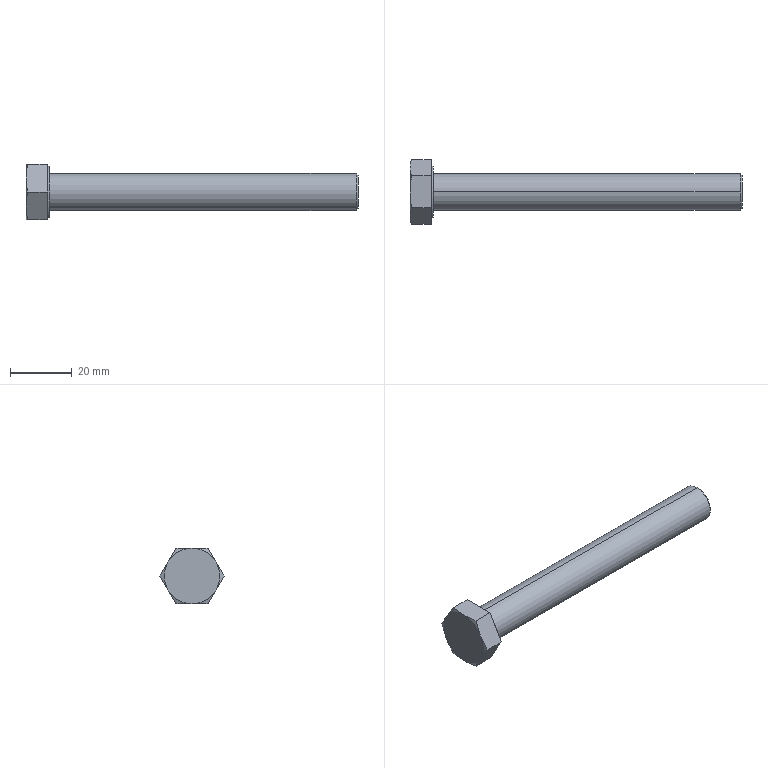Part | STEP file | GBT 5781#Hex head bolt fully threaded_M12×100-zinc plated | 1 solid | 22 faces | box 107.5 x 20.785 x 18 mm | volume 13373 mm3 | cone 10 | plane 10 | cylinder 2 | commonest cylinder face diameters 12 x2
STEP:
#1=CARTESIAN_POINT('',(107.5,0.,-5.4));
#2=VERTEX_POINT('',#1);
#3=CARTESIAN_POINT('',(107.5,0.,5.4));
#4=VERTEX_POINT('',#3);
#5=CARTESIAN_POINT('',(107.5,0.,0.));
#6=DIRECTION('',(1.,0.,0.));
#7=DIRECTION('',(0.,0.,-1.));
#8=AXIS2_PLACEMENT_3D('',#5,#6,#7);
#9=CIRCLE('',#8,5.4);
#10=EDGE_CURVE('',#2,#4,#9,.T.);
#11=ORIENTED_EDGE('',*,*,#10,.F.);
#12=CARTESIAN_POINT('',(106.9,0.,-6.));
#13=VERTEX_POINT('',#12);
#14=CARTESIAN_POINT('',(107.5,0.,-5.4));
#15=DIRECTION('',(-0.7071,0.,-0.7071));
#16=VECTOR('',#15,1000.);
#17=LINE('',#14,#16);
#18=EDGE_CURVE('',#2,#13,#17,.T.);
#19=ORIENTED_EDGE('',*,*,#18,.T.);
#20=CARTESIAN_POINT('',(106.9,0.,6.));
#21=VERTEX_POINT('',#20);
#22=CARTESIAN_POINT('',(106.9,0.,0.));
#23=DIRECTION('',(-1.,0.,0.));
#24=DIRECTION('',(0.,0.,-1.));
#25=AXIS2_PLACEMENT_3D('',#22,#23,#24);
#26=CIRCLE('',#25,6.);
#27=EDGE_CURVE('',#21,#13,#26,.T.);
#28=ORIENTED_EDGE('',*,*,#27,.F.);
#29=CARTESIAN_POINT('',(107.5,0.,5.4));
#30=DIRECTION('',(-0.7071,0.,0.7071));
#31=VECTOR('',#30,1000.);
#32=LINE('',#29,#31);
#33=EDGE_CURVE('',#4,#21,#32,.T.);
#34=ORIENTED_EDGE('',*,*,#33,.F.);
#35=EDGE_LOOP('',(#11,#19,#28,#34));
#36=FACE_OUTER_BOUND('',#35,.T.);
#37=CARTESIAN_POINT('',(107.5,0.,0.));
#38=DIRECTION('',(-1.,0.,0.));
#39=DIRECTION('',(0.,0.,1.));
#40=AXIS2_PLACEMENT_3D('',#37,#38,#39);
#41=CONICAL_SURFACE('',#40,5.4,0.7854);
#42=ADVANCED_FACE('',(#36),#41,.T.);
#43=ORIENTED_EDGE('',*,*,#27,.T.);
#44=CARTESIAN_POINT('',(7.5,0.,-6.));
#45=VERTEX_POINT('',#44);
#46=CARTESIAN_POINT('',(107.5,0.,-6.));
#47=DIRECTION('',(-1.,0.,0.));
#48=VECTOR('',#47,1000.);
#49=LINE('',#46,#48);
#50=EDGE_CURVE('',#13,#45,#49,.T.);
#51=ORIENTED_EDGE('',*,*,#50,.T.);
#52=CARTESIAN_POINT('',(7.5,0.,6.));
#53=VERTEX_POINT('',#52);
#54=CARTESIAN_POINT('',(7.5,0.,0.));
#55=DIRECTION('',(1.,0.,0.));
#56=DIRECTION('',(0.,0.,-1.));
#57=AXIS2_PLACEMENT_3D('',#54,#55,#56);
#58=CIRCLE('',#57,6.);
#59=EDGE_CURVE('',#45,#53,#58,.T.);
#60=ORIENTED_EDGE('',*,*,#59,.T.);
#61=CARTESIAN_POINT('',(107.5,0.,6.));
#62=DIRECTION('',(-1.,0.,0.));
#63=VECTOR('',#62,1000.);
#64=LINE('',#61,#63);
#65=EDGE_CURVE('',#21,#53,#64,.T.);
#66=ORIENTED_EDGE('',*,*,#65,.F.);
#67=EDGE_LOOP('',(#43,#51,#60,#66));
#68=FACE_OUTER_BOUND('',#67,.T.);
#69=CARTESIAN_POINT('',(107.5,0.,0.));
#70=DIRECTION('',(-1.,0.,0.));
#71=DIRECTION('',(0.,0.,1.));
#72=AXIS2_PLACEMENT_3D('',#69,#70,#71);
#73=CYLINDRICAL_SURFACE('',#72,6.);
#74=ADVANCED_FACE('',(#68),#73,.T.);
#75=CARTESIAN_POINT('',(7.5,0.,8.235));
#76=VERTEX_POINT('',#75);
#77=CARTESIAN_POINT('',(7.5,0.,-8.235));
#78=VERTEX_POINT('',#77);
#79=CARTESIAN_POINT('',(7.5,0.,0.));
#80=DIRECTION('',(-1.,0.,0.));
#81=DIRECTION('',(0.,0.,1.));
#82=AXIS2_PLACEMENT_3D('',#79,#80,#81);
#83=CIRCLE('',#82,8.235);
#84=EDGE_CURVE('',#76,#78,#83,.T.);
#85=ORIENTED_EDGE('',*,*,#84,.T.);
#86=CARTESIAN_POINT('',(6.9,0.,-8.835));
#87=VERTEX_POINT('',#86);
#88=CARTESIAN_POINT('',(6.9,0.,-8.835));
#89=DIRECTION('',(-0.7071,0.,-0.7071));
#90=VECTOR('',#89,1000.);
#91=LINE('',#88,#90);
#92=EDGE_CURVE('',#78,#87,#91,.T.);
#93=ORIENTED_EDGE('',*,*,#92,.T.);
#94=CARTESIAN_POINT('',(6.9,0.,8.835));
#95=VERTEX_POINT('',#94);
#96=CARTESIAN_POINT('',(6.9,0.,0.));
#97=DIRECTION('',(-1.,0.,0.));
#98=DIRECTION('',(0.,0.,1.));
#99=AXIS2_PLACEMENT_3D('',#96,#97,#98);
#100=CIRCLE('',#99,8.835);
#101=EDGE_CURVE('',#95,#87,#100,.T.);
#102=ORIENTED_EDGE('',*,*,#101,.F.);
#103=CARTESIAN_POINT('',(6.9,0.,8.835));
#104=DIRECTION('',(-0.7071,0.,0.7071));
#105=VECTOR('',#104,1000.);
#106=LINE('',#103,#105);
#107=EDGE_CURVE('',#76,#95,#106,.T.);
#108=ORIENTED_EDGE('',*,*,#107,.F.);
#109=EDGE_LOOP('',(#85,#93,#102,#108));
#110=FACE_OUTER_BOUND('',#109,.T.);
#111=CARTESIAN_POINT('',(6.9,0.,0.));
#112=DIRECTION('',(-1.,0.,0.));
#113=DIRECTION('',(0.,0.,1.));
#114=AXIS2_PLACEMENT_3D('',#111,#112,#113);
#115=CONICAL_SURFACE('',#114,8.835,0.7854);
#116=ADVANCED_FACE('',(#110),#115,.T.);
#117=ORIENTED_EDGE('',*,*,#84,.F.);
#118=CARTESIAN_POINT('',(7.5,0.,0.));
#119=DIRECTION('',(-1.,0.,0.));
#120=DIRECTION('',(0.,0.,1.));
#121=AXIS2_PLACEMENT_3D('',#118,#119,#120);
#122=CIRCLE('',#121,8.235);
#123=EDGE_CURVE('',#78,#76,#122,.T.);
#124=ORIENTED_EDGE('',*,*,#123,.F.);
#125=EDGE_LOOP('',(#117,#124));
#126=FACE_OUTER_BOUND('',#125,.T.);
#127=CARTESIAN_POINT('',(7.5,0.,0.));
#128=DIRECTION('',(1.,0.,0.));
#129=DIRECTION('',(0.,0.,-1.));
#130=AXIS2_PLACEMENT_3D('',#127,#128,#129);
#131=CIRCLE('',#130,6.);
#132=EDGE_CURVE('',#53,#45,#131,.T.);
#133=ORIENTED_EDGE('',*,*,#132,.F.);
#134=ORIENTED_EDGE('',*,*,#59,.F.);
#135=EDGE_LOOP('',(#133,#134));
#136=FACE_BOUND('',#135,.T.);
#137=CARTESIAN_POINT('',(7.5,-10.392,0.));
#138=DIRECTION('',(1.,0.,0.));
#139=DIRECTION('',(0.,0.,-1.));
#140=AXIS2_PLACEMENT_3D('',#137,#138,#139);
#141=PLANE('',#140);
#142=ADVANCED_FACE('',(#126,#136),#141,.T.);
#143=CARTESIAN_POINT('',(0.5068,-10.392,0.));
#144=VERTEX_POINT('',#143);
#145=CARTESIAN_POINT('',(0.,-7.794,4.5));
#146=VERTEX_POINT('',#145);
#147=CARTESIAN_POINT('',(0.5068,-10.392,0.));
#148=CARTESIAN_POINT('',(0.3492,-9.959,0.75));
#149=CARTESIAN_POINT('',(0.2212,-9.526,1.5));
#150=CARTESIAN_POINT('',(0.04634,-8.66,3.));
#151=CARTESIAN_POINT('',(0.,-8.227,3.75));
#152=CARTESIAN_POINT('',(0.,-7.794,4.5));
#153=B_SPLINE_CURVE_WITH_KNOTS('',3,(#147,#148,#149,#150,#151,#152),.UNSPECIFIED.,.F.,.F.,(4,2,4),(0.000000231,0.002598,0.005196),.UNSPECIFIED.);
#154=EDGE_CURVE('',#144,#146,#153,.T.);
#155=ORIENTED_EDGE('',*,*,#154,.F.);
#156=CARTESIAN_POINT('',(6.9,-10.392,0.));
#157=VERTEX_POINT('',#156);
#158=CARTESIAN_POINT('',(7.5,-10.392,0.));
#159=DIRECTION('',(-1.,0.,0.));
#160=VECTOR('',#159,1000.);
#161=LINE('',#158,#160);
#162=EDGE_CURVE('',#157,#144,#161,.T.);
#163=ORIENTED_EDGE('',*,*,#162,.F.);
#164=CARTESIAN_POINT('',(6.9,-5.196,9.));
#165=VERTEX_POINT('',#164);
#166=CARTESIAN_POINT('',(6.9,-5.196,9.));
#167=DIRECTION('',(0.,-0.5,-0.866));
#168=VECTOR('',#167,1000.);
#169=LINE('',#166,#168);
#170=EDGE_CURVE('',#165,#157,#169,.T.);
#171=ORIENTED_EDGE('',*,*,#170,.F.);
#172=CARTESIAN_POINT('',(0.5068,-5.196,9.));
#173=VERTEX_POINT('',#172);
#174=CARTESIAN_POINT('',(7.5,-5.196,9.));
#175=DIRECTION('',(-1.,0.,0.));
#176=VECTOR('',#175,1000.);
#177=LINE('',#174,#176);
#178=EDGE_CURVE('',#165,#173,#177,.T.);
#179=ORIENTED_EDGE('',*,*,#178,.T.);
#180=CARTESIAN_POINT('',(0.,-7.794,4.5));
#181=CARTESIAN_POINT('',(0.,-7.361,5.25));
#182=CARTESIAN_POINT('',(0.04634,-6.928,6.));
#183=CARTESIAN_POINT('',(0.2212,-6.062,7.5));
#184=CARTESIAN_POINT('',(0.3492,-5.629,8.25));
#185=CARTESIAN_POINT('',(0.5068,-5.196,9.));
#186=B_SPLINE_CURVE_WITH_KNOTS('',3,(#180,#181,#182,#183,#184,#185),.UNSPECIFIED.,.F.,.F.,(4,2,4),(0.005196,0.007794,0.01039),.UNSPECIFIED.);
#187=EDGE_CURVE('',#146,#173,#186,.T.);
#188=ORIENTED_EDGE('',*,*,#187,.F.);
#189=EDGE_LOOP('',(#155,#163,#171,#179,#188));
#190=FACE_OUTER_BOUND('',#189,.T.);
#191=CARTESIAN_POINT('',(7.5,-5.196,9.));
#192=DIRECTION('',(0.,0.866,-0.5));
#193=DIRECTION('',(0.,0.5,0.866));
#194=AXIS2_PLACEMENT_3D('',#191,#192,#193);
#195=PLANE('',#194);
#196=ADVANCED_FACE('',(#190),#195,.F.);
#197=CARTESIAN_POINT('',(0.5068,-5.196,-9.));
#198=VERTEX_POINT('',#197);
#199=CARTESIAN_POINT('',(0.,-7.794,-4.5));
#200=VERTEX_POINT('',#199);
#201=CARTESIAN_POINT('',(0.5068,-5.196,-9.));
#202=CARTESIAN_POINT('',(0.3492,-5.629,-8.25));
#203=CARTESIAN_POINT('',(0.2212,-6.062,-7.5));
#204=CARTESIAN_POINT('',(0.04634,-6.928,-6.));
#205=CARTESIAN_POINT('',(0.,-7.361,-5.25));
#206=CARTESIAN_POINT('',(0.,-7.794,-4.5));
#207=B_SPLINE_CURVE_WITH_KNOTS('',3,(#201,#202,#203,#204,#205,#206),.UNSPECIFIED.,.F.,.F.,(4,2,4),(0.000000231,0.002598,0.005196),.UNSPECIFIED.);
#208=EDGE_CURVE('',#198,#200,#207,.T.);
#209=ORIENTED_EDGE('',*,*,#208,.F.);
#210=CARTESIAN_POINT('',(6.9,-5.196,-9.));
#211=VERTEX_POINT('',#210);
#212=CARTESIAN_POINT('',(7.5,-5.196,-9.));
#213=DIRECTION('',(-1.,0.,0.));
#214=VECTOR('',#213,1000.);
#215=LINE('',#212,#214);
#216=EDGE_CURVE('',#211,#198,#215,.T.);
#217=ORIENTED_EDGE('',*,*,#216,.F.);
#218=CARTESIAN_POINT('',(6.9,-10.392,0.));
#219=DIRECTION('',(0.,0.5,-0.866));
#220=VECTOR('',#219,1000.);
#221=LINE('',#218,#220);
#222=EDGE_CURVE('',#157,#211,#221,.T.);
#223=ORIENTED_EDGE('',*,*,#222,.F.);
#224=ORIENTED_EDGE('',*,*,#162,.T.);
#225=CARTESIAN_POINT('',(0.,-7.794,-4.5));
#226=CARTESIAN_POINT('',(0.,-8.227,-3.75));
#227=CARTESIAN_POINT('',(0.04634,-8.66,-3.));
#228=CARTESIAN_POINT('',(0.2212,-9.526,-1.5));
#229=CARTESIAN_POINT('',(0.3492,-9.959,-0.75));
#230=CARTESIAN_POINT('',(0.5068,-10.392,0.));
#231=B_SPLINE_CURVE_WITH_KNOTS('',3,(#225,#226,#227,#228,#229,#230),.UNSPECIFIED.,.F.,.F.,(4,2,4),(0.005196,0.007794,0.01039),.UNSPECIFIED.);
#232=EDGE_CURVE('',#200,#144,#231,.T.);
#233=ORIENTED_EDGE('',*,*,#232,.F.);
#234=EDGE_LOOP('',(#209,#217,#223,#224,#233));
#235=FACE_OUTER_BOUND('',#234,.T.);
#236=CARTESIAN_POINT('',(7.5,-10.392,0.));
#237=DIRECTION('',(0.,0.866,0.5));
#238=DIRECTION('',(0.,-0.5,0.866));
#239=AXIS2_PLACEMENT_3D('',#236,#237,#238);
#240=PLANE('',#239);
#241=ADVANCED_FACE('',(#235),#240,.F.);
#242=CARTESIAN_POINT('',(0.5068,5.196,-9.));
#243=VERTEX_POINT('',#242);
#244=CARTESIAN_POINT('',(0.,0.,-9.));
#245=VERTEX_POINT('',#244);
#246=CARTESIAN_POINT('',(0.5068,5.196,-9.));
#247=CARTESIAN_POINT('',(0.3496,4.332,-9.));
#248=CARTESIAN_POINT('',(0.2215,3.467,-9.));
#249=CARTESIAN_POINT('',(0.04652,1.735,-9.));
#250=CARTESIAN_POINT('',(0.,0.8678,-9.));
#251=CARTESIAN_POINT('',(0.,0.,-9.));
#252=B_SPLINE_CURVE_WITH_KNOTS('',3,(#246,#247,#248,#249,#250,#251),.UNSPECIFIED.,.F.,.F.,(4,2,4),(0.01874,0.02136,0.02398),.UNSPECIFIED.);
#253=EDGE_CURVE('',#243,#245,#252,.T.);
#254=ORIENTED_EDGE('',*,*,#253,.F.);
#255=CARTESIAN_POINT('',(6.9,5.196,-9.));
#256=VERTEX_POINT('',#255);
#257=CARTESIAN_POINT('',(7.5,5.196,-9.));
#258=DIRECTION('',(-1.,0.,0.));
#259=VECTOR('',#258,1000.);
#260=LINE('',#257,#259);
#261=EDGE_CURVE('',#256,#243,#260,.T.);
#262=ORIENTED_EDGE('',*,*,#261,.F.);
#263=CARTESIAN_POINT('',(6.9,-5.196,-9.));
#264=DIRECTION('',(0.,1.,0.));
#265=VECTOR('',#264,1000.);
#266=LINE('',#263,#265);
#267=EDGE_CURVE('',#211,#256,#266,.T.);
#268=ORIENTED_EDGE('',*,*,#267,.F.);
#269=ORIENTED_EDGE('',*,*,#216,.T.);
#270=CARTESIAN_POINT('',(0.,0.,-9.));
#271=CARTESIAN_POINT('',(0.,-0.8653,-9.));
#272=CARTESIAN_POINT('',(0.04627,-1.732,-9.));
#273=CARTESIAN_POINT('',(0.2214,-3.466,-9.));
#274=CARTESIAN_POINT('',(0.3502,-4.336,-9.));
#275=CARTESIAN_POINT('',(0.5068,-5.196,-9.));
#276=B_SPLINE_CURVE_WITH_KNOTS('',3,(#270,#271,#272,#273,#274,#275),.UNSPECIFIED.,.F.,.F.,(4,2,4),(0.02398,0.02659,0.0292),.UNSPECIFIED.);
#277=EDGE_CURVE('',#245,#198,#276,.T.);
#278=ORIENTED_EDGE('',*,*,#277,.F.);
#279=EDGE_LOOP('',(#254,#262,#268,#269,#278));
#280=FACE_OUTER_BOUND('',#279,.T.);
#281=CARTESIAN_POINT('',(7.5,-5.196,-9.));
#282=DIRECTION('',(0.,0.,1.));
#283=DIRECTION('',(1.,0.,0.));
#284=AXIS2_PLACEMENT_3D('',#281,#282,#283);
#285=PLANE('',#284);
#286=ADVANCED_FACE('',(#280),#285,.F.);
#287=CARTESIAN_POINT('',(0.5068,10.392,0.));
#288=VERTEX_POINT('',#287);
#289=CARTESIAN_POINT('',(0.,7.794,-4.5));
#290=VERTEX_POINT('',#289);
#291=CARTESIAN_POINT('',(0.5068,10.392,0.));
#292=CARTESIAN_POINT('',(0.3492,9.959,-0.75));
#293=CARTESIAN_POINT('',(0.2212,9.526,-1.5));
#294=CARTESIAN_POINT('',(0.04634,8.66,-3.));
#295=CARTESIAN_POINT('',(0.,8.227,-3.75));
#296=CARTESIAN_POINT('',(0.,7.794,-4.5));
#297=B_SPLINE_CURVE_WITH_KNOTS('',3,(#291,#292,#293,#294,#295,#296),.UNSPECIFIED.,.F.,.F.,(4,2,4),(0.000000231,0.002598,0.005196),.UNSPECIFIED.);
#298=EDGE_CURVE('',#288,#290,#297,.T.);
#299=ORIENTED_EDGE('',*,*,#298,.F.);
#300=CARTESIAN_POINT('',(6.9,10.392,0.));
#301=VERTEX_POINT('',#300);
#302=CARTESIAN_POINT('',(7.5,10.392,0.));
#303=DIRECTION('',(-1.,0.,0.));
#304=VECTOR('',#303,1000.);
#305=LINE('',#302,#304);
#306=EDGE_CURVE('',#301,#288,#305,.T.);
#307=ORIENTED_EDGE('',*,*,#306,.F.);
#308=CARTESIAN_POINT('',(6.9,5.196,-9.));
#309=DIRECTION('',(0.,0.5,0.866));
#310=VECTOR('',#309,1000.);
#311=LINE('',#308,#310);
#312=EDGE_CURVE('',#256,#301,#311,.T.);
#313=ORIENTED_EDGE('',*,*,#312,.F.);
#314=ORIENTED_EDGE('',*,*,#261,.T.);
#315=CARTESIAN_POINT('',(0.,7.794,-4.5));
#316=CARTESIAN_POINT('',(0.,7.361,-5.25));
#317=CARTESIAN_POINT('',(0.04634,6.928,-6.));
#318=CARTESIAN_POINT('',(0.2212,6.062,-7.5));
#319=CARTESIAN_POINT('',(0.3492,5.629,-8.25));
#320=CARTESIAN_POINT('',(0.5068,5.196,-9.));
#321=B_SPLINE_CURVE_WITH_KNOTS('',3,(#315,#316,#317,#318,#319,#320),.UNSPECIFIED.,.F.,.F.,(4,2,4),(0.005196,0.007794,0.01039),.UNSPECIFIED.);
#322=EDGE_CURVE('',#290,#243,#321,.T.);
#323=ORIENTED_EDGE('',*,*,#322,.F.);
#324=EDGE_LOOP('',(#299,#307,#313,#314,#323));
#325=FACE_OUTER_BOUND('',#324,.T.);
#326=CARTESIAN_POINT('',(7.5,5.196,-9.));
#327=DIRECTION('',(0.,-0.866,0.5));
#328=DIRECTION('',(0.,-0.5,-0.866));
#329=AXIS2_PLACEMENT_3D('',#326,#327,#328);
#330=PLANE('',#329);
#331=ADVANCED_FACE('',(#325),#330,.F.);
#332=CARTESIAN_POINT('',(0.5068,5.196,9.));
#333=VERTEX_POINT('',#332);
#334=CARTESIAN_POINT('',(0.,7.794,4.5));
#335=VERTEX_POINT('',#334);
#336=CARTESIAN_POINT('',(0.5068,5.196,9.));
#337=CARTESIAN_POINT('',(0.3492,5.629,8.25));
#338=CARTESIAN_POINT('',(0.2212,6.062,7.5));
#339=CARTESIAN_POINT('',(0.04634,6.928,6.));
#340=CARTESIAN_POINT('',(0.,7.361,5.25));
#341=CARTESIAN_POINT('',(0.,7.794,4.5));
#342=B_SPLINE_CURVE_WITH_KNOTS('',3,(#336,#337,#338,#339,#340,#341),.UNSPECIFIED.,.F.,.F.,(4,2,4),(0.000000231,0.002598,0.005196),.UNSPECIFIED.);
#343=EDGE_CURVE('',#333,#335,#342,.T.);
#344=ORIENTED_EDGE('',*,*,#343,.F.);
#345=CARTESIAN_POINT('',(6.9,5.196,9.));
#346=VERTEX_POINT('',#345);
#347=CARTESIAN_POINT('',(7.5,5.196,9.));
#348=DIRECTION('',(-1.,0.,0.));
#349=VECTOR('',#348,1000.);
#350=LINE('',#347,#349);
#351=EDGE_CURVE('',#346,#333,#350,.T.);
#352=ORIENTED_EDGE('',*,*,#351,.F.);
#353=CARTESIAN_POINT('',(6.9,10.392,0.));
#354=DIRECTION('',(0.,-0.5,0.866));
#355=VECTOR('',#354,1000.);
#356=LINE('',#353,#355);
#357=EDGE_CURVE('',#301,#346,#356,.T.);
#358=ORIENTED_EDGE('',*,*,#357,.F.);
#359=ORIENTED_EDGE('',*,*,#306,.T.);
#360=CARTESIAN_POINT('',(0.,7.794,4.5));
#361=CARTESIAN_POINT('',(0.,8.227,3.75));
#362=CARTESIAN_POINT('',(0.04634,8.66,3.));
#363=CARTESIAN_POINT('',(0.2212,9.526,1.5));
#364=CARTESIAN_POINT('',(0.3492,9.959,0.75));
#365=CARTESIAN_POINT('',(0.5068,10.392,0.));
#366=B_SPLINE_CURVE_WITH_KNOTS('',3,(#360,#361,#362,#363,#364,#365),.UNSPECIFIED.,.F.,.F.,(4,2,4),(0.005196,0.007794,0.01039),.UNSPECIFIED.);
#367=EDGE_CURVE('',#335,#288,#366,.T.);
#368=ORIENTED_EDGE('',*,*,#367,.F.);
#369=EDGE_LOOP('',(#344,#352,#358,#359,#368));
#370=FACE_OUTER_BOUND('',#369,.T.);
#371=CARTESIAN_POINT('',(7.5,10.392,0.));
#372=DIRECTION('',(0.,-0.866,-0.5));
#373=DIRECTION('',(0.,0.5,-0.866));
#374=AXIS2_PLACEMENT_3D('',#371,#372,#373);
#375=PLANE('',#374);
#376=ADVANCED_FACE('',(#370),#375,.F.);
#377=CARTESIAN_POINT('',(0.,0.,9.));
#378=VERTEX_POINT('',#377);
#379=CARTESIAN_POINT('',(0.5068,-5.196,9.));
#380=CARTESIAN_POINT('',(0.3502,-4.336,9.));
#381=CARTESIAN_POINT('',(0.2214,-3.466,9.));
#382=CARTESIAN_POINT('',(0.04627,-1.732,9.));
#383=CARTESIAN_POINT('',(0.,-0.8653,9.));
#384=CARTESIAN_POINT('',(0.,0.,9.));
#385=B_SPLINE_CURVE_WITH_KNOTS('',3,(#379,#380,#381,#382,#383,#384),.UNSPECIFIED.,.F.,.F.,(4,2,4),(0.008839,0.01146,0.01408),.UNSPECIFIED.);
#386=EDGE_CURVE('',#173,#378,#385,.T.);
#387=ORIENTED_EDGE('',*,*,#386,.F.);
#388=ORIENTED_EDGE('',*,*,#178,.F.);
#389=CARTESIAN_POINT('',(6.9,5.196,9.));
#390=DIRECTION('',(0.,-1.,0.));
#391=VECTOR('',#390,1000.);
#392=LINE('',#389,#391);
#393=EDGE_CURVE('',#346,#165,#392,.T.);
#394=ORIENTED_EDGE('',*,*,#393,.F.);
#395=ORIENTED_EDGE('',*,*,#351,.T.);
#396=CARTESIAN_POINT('',(0.,0.,9.));
#397=CARTESIAN_POINT('',(0.,0.8678,9.));
#398=CARTESIAN_POINT('',(0.04652,1.735,9.));
#399=CARTESIAN_POINT('',(0.2215,3.467,9.));
#400=CARTESIAN_POINT('',(0.3496,4.332,9.));
#401=CARTESIAN_POINT('',(0.5068,5.196,9.));
#402=B_SPLINE_CURVE_WITH_KNOTS('',3,(#396,#397,#398,#399,#400,#401),.UNSPECIFIED.,.F.,.F.,(4,2,4),(0.01408,0.0167,0.01933),.UNSPECIFIED.);
#403=EDGE_CURVE('',#378,#333,#402,.T.);
#404=ORIENTED_EDGE('',*,*,#403,.F.);
#405=EDGE_LOOP('',(#387,#388,#394,#395,#404));
#406=FACE_OUTER_BOUND('',#405,.T.);
#407=CARTESIAN_POINT('',(7.5,5.196,9.));
#408=DIRECTION('',(0.,0.,-1.));
#409=DIRECTION('',(-1.,0.,0.));
#410=AXIS2_PLACEMENT_3D('',#407,#408,#409);
#411=PLANE('',#410);
#412=ADVANCED_FACE('',(#406),#411,.F.);
#413=ORIENTED_EDGE('',*,*,#101,.T.);
#414=CARTESIAN_POINT('',(6.9,0.,0.));
#415=DIRECTION('',(-1.,0.,0.));
#416=DIRECTION('',(0.,0.,1.));
#417=AXIS2_PLACEMENT_3D('',#414,#415,#416);
#418=CIRCLE('',#417,8.835);
#419=EDGE_CURVE('',#87,#95,#418,.T.);
#420=ORIENTED_EDGE('',*,*,#419,.T.);
#421=EDGE_LOOP('',(#413,#420));
#422=FACE_BOUND('',#421,.T.);
#423=ORIENTED_EDGE('',*,*,#170,.T.);
#424=ORIENTED_EDGE('',*,*,#222,.T.);
#425=ORIENTED_EDGE('',*,*,#267,.T.);
#426=ORIENTED_EDGE('',*,*,#312,.T.);
#427=ORIENTED_EDGE('',*,*,#357,.T.);
#428=ORIENTED_EDGE('',*,*,#393,.T.);
#429=EDGE_LOOP('',(#423,#424,#425,#426,#427,#428));
#430=FACE_OUTER_BOUND('',#429,.T.);
#431=CARTESIAN_POINT('',(6.9,8.835,0.));
#432=DIRECTION('',(1.,0.,0.));
#433=DIRECTION('',(0.,0.,-1.));
#434=AXIS2_PLACEMENT_3D('',#431,#432,#433);
#435=PLANE('',#434);
#436=ADVANCED_FACE('',(#422,#430),#435,.T.);
#437=ORIENTED_EDGE('',*,*,#92,.F.);
#438=ORIENTED_EDGE('',*,*,#123,.T.);
#439=ORIENTED_EDGE('',*,*,#107,.T.);
#440=ORIENTED_EDGE('',*,*,#419,.F.);
#441=EDGE_LOOP('',(#437,#438,#439,#440));
#442=FACE_OUTER_BOUND('',#441,.T.);
#443=CARTESIAN_POINT('',(6.9,0.,0.));
#444=DIRECTION('',(-1.,0.,0.));
#445=DIRECTION('',(0.,0.,1.));
#446=AXIS2_PLACEMENT_3D('',#443,#444,#445);
#447=CONICAL_SURFACE('',#446,8.835,0.7854);
#448=ADVANCED_FACE('',(#442),#447,.T.);
#449=ORIENTED_EDGE('',*,*,#277,.T.);
#450=ORIENTED_EDGE('',*,*,#208,.T.);
#451=CARTESIAN_POINT('',(0.,0.,0.));
#452=DIRECTION('',(1.,0.,0.));
#453=DIRECTION('',(0.,0.,-1.));
#454=AXIS2_PLACEMENT_3D('',#451,#452,#453);
#455=CIRCLE('',#454,9.);
#456=EDGE_CURVE('',#200,#245,#455,.T.);
#457=ORIENTED_EDGE('',*,*,#456,.T.);
#458=EDGE_LOOP('',(#449,#450,#457));
#459=FACE_OUTER_BOUND('',#458,.T.);
#460=CARTESIAN_POINT('',(0.,0.,0.));
#461=DIRECTION('',(1.,0.,0.));
#462=DIRECTION('',(0.,0.,-1.));
#463=AXIS2_PLACEMENT_3D('',#460,#461,#462);
#464=CONICAL_SURFACE('',#463,9.,1.222);
#465=ADVANCED_FACE('',(#459),#464,.T.);
#466=ORIENTED_EDGE('',*,*,#232,.T.);
#467=ORIENTED_EDGE('',*,*,#154,.T.);
#468=CARTESIAN_POINT('',(0.,0.,0.));
#469=DIRECTION('',(1.,0.,0.));
#470=DIRECTION('',(0.,0.,-1.));
#471=AXIS2_PLACEMENT_3D('',#468,#469,#470);
#472=CIRCLE('',#471,9.);
#473=EDGE_CURVE('',#146,#200,#472,.T.);
#474=ORIENTED_EDGE('',*,*,#473,.T.);
#475=EDGE_LOOP('',(#466,#467,#474));
#476=FACE_OUTER_BOUND('',#475,.T.);
#477=CARTESIAN_POINT('',(0.,0.,0.));
#478=DIRECTION('',(1.,0.,0.));
#479=DIRECTION('',(0.,0.,-1.));
#480=AXIS2_PLACEMENT_3D('',#477,#478,#479);
#481=CONICAL_SURFACE('',#480,9.,1.222);
#482=ADVANCED_FACE('',(#476),#481,.T.);
#483=ORIENTED_EDGE('',*,*,#187,.T.);
#484=ORIENTED_EDGE('',*,*,#386,.T.);
#485=CARTESIAN_POINT('',(0.,0.,0.));
#486=DIRECTION('',(1.,0.,0.));
#487=DIRECTION('',(0.,0.,-1.));
#488=AXIS2_PLACEMENT_3D('',#485,#486,#487);
#489=CIRCLE('',#488,9.);
#490=EDGE_CURVE('',#378,#146,#489,.T.);
#491=ORIENTED_EDGE('',*,*,#490,.T.);
#492=EDGE_LOOP('',(#483,#484,#491));
#493=FACE_OUTER_BOUND('',#492,.T.);
#494=CARTESIAN_POINT('',(0.,0.,0.));
#495=DIRECTION('',(1.,0.,0.));
#496=DIRECTION('',(0.,0.,-1.));
#497=AXIS2_PLACEMENT_3D('',#494,#495,#496);
#498=CONICAL_SURFACE('',#497,9.,1.222);
#499=ADVANCED_FACE('',(#493),#498,.T.);
#500=ORIENTED_EDGE('',*,*,#343,.T.);
#501=CARTESIAN_POINT('',(0.,0.,0.));
#502=DIRECTION('',(-1.,0.,0.));
#503=DIRECTION('',(0.,0.,1.));
#504=AXIS2_PLACEMENT_3D('',#501,#502,#503);
#505=CIRCLE('',#504,9.);
#506=EDGE_CURVE('',#378,#335,#505,.T.);
#507=ORIENTED_EDGE('',*,*,#506,.F.);
#508=ORIENTED_EDGE('',*,*,#403,.T.);
#509=EDGE_LOOP('',(#500,#507,#508));
#510=FACE_OUTER_BOUND('',#509,.T.);
#511=CARTESIAN_POINT('',(0.,0.,0.));
#512=DIRECTION('',(1.,0.,0.));
#513=DIRECTION('',(0.,0.,-1.));
#514=AXIS2_PLACEMENT_3D('',#511,#512,#513);
#515=CONICAL_SURFACE('',#514,9.,1.222);
#516=ADVANCED_FACE('',(#510),#515,.T.);
#517=ORIENTED_EDGE('',*,*,#298,.T.);
#518=CARTESIAN_POINT('',(0.,0.,0.));
#519=DIRECTION('',(1.,0.,0.));
#520=DIRECTION('',(0.,0.,-1.));
#521=AXIS2_PLACEMENT_3D('',#518,#519,#520);
#522=CIRCLE('',#521,9.);
#523=EDGE_CURVE('',#290,#335,#522,.T.);
#524=ORIENTED_EDGE('',*,*,#523,.T.);
#525=ORIENTED_EDGE('',*,*,#367,.T.);
#526=EDGE_LOOP('',(#517,#524,#525));
#527=FACE_OUTER_BOUND('',#526,.T.);
#528=CARTESIAN_POINT('',(0.,0.,0.));
#529=DIRECTION('',(1.,0.,0.));
#530=DIRECTION('',(0.,0.,-1.));
#531=AXIS2_PLACEMENT_3D('',#528,#529,#530);
#532=CONICAL_SURFACE('',#531,9.,1.222);
#533=ADVANCED_FACE('',(#527),#532,.T.);
#534=ORIENTED_EDGE('',*,*,#253,.T.);
#535=CARTESIAN_POINT('',(0.,0.,0.));
#536=DIRECTION('',(1.,0.,0.));
#537=DIRECTION('',(0.,0.,-1.));
#538=AXIS2_PLACEMENT_3D('',#535,#536,#537);
#539=CIRCLE('',#538,9.);
#540=EDGE_CURVE('',#245,#290,#539,.T.);
#541=ORIENTED_EDGE('',*,*,#540,.T.);
#542=ORIENTED_EDGE('',*,*,#322,.T.);
#543=EDGE_LOOP('',(#534,#541,#542));
#544=FACE_OUTER_BOUND('',#543,.T.);
#545=CARTESIAN_POINT('',(0.,0.,0.));
#546=DIRECTION('',(1.,0.,0.));
#547=DIRECTION('',(0.,0.,-1.));
#548=AXIS2_PLACEMENT_3D('',#545,#546,#547);
#549=CONICAL_SURFACE('',#548,9.,1.222);
#550=ADVANCED_FACE('',(#544),#549,.T.);
#551=ORIENTED_EDGE('',*,*,#540,.F.);
#552=ORIENTED_EDGE('',*,*,#456,.F.);
#553=ORIENTED_EDGE('',*,*,#473,.F.);
#554=ORIENTED_EDGE('',*,*,#490,.F.);
#555=ORIENTED_EDGE('',*,*,#506,.T.);
#556=ORIENTED_EDGE('',*,*,#523,.F.);
#557=EDGE_LOOP('',(#551,#552,#553,#554,#555,#556));
#558=FACE_OUTER_BOUND('',#557,.T.);
#559=CARTESIAN_POINT('',(0.,-10.392,0.));
#560=DIRECTION('',(1.,0.,0.));
#561=DIRECTION('',(0.,0.,-1.));
#562=AXIS2_PLACEMENT_3D('',#559,#560,#561);
#563=PLANE('',#562);
#564=ADVANCED_FACE('',(#558),#563,.F.);
#565=ORIENTED_EDGE('',*,*,#50,.F.);
#566=CARTESIAN_POINT('',(106.9,0.,0.));
#567=DIRECTION('',(-1.,0.,0.));
#568=DIRECTION('',(0.,0.,-1.));
#569=AXIS2_PLACEMENT_3D('',#566,#567,#568);
#570=CIRCLE('',#569,6.);
#571=EDGE_CURVE('',#13,#21,#570,.T.);
#572=ORIENTED_EDGE('',*,*,#571,.T.);
#573=ORIENTED_EDGE('',*,*,#65,.T.);
#574=ORIENTED_EDGE('',*,*,#132,.T.);
#575=EDGE_LOOP('',(#565,#572,#573,#574));
#576=FACE_OUTER_BOUND('',#575,.T.);
#577=CARTESIAN_POINT('',(107.5,0.,0.));
#578=DIRECTION('',(-1.,0.,0.));
#579=DIRECTION('',(0.,0.,1.));
#580=AXIS2_PLACEMENT_3D('',#577,#578,#579);
#581=CYLINDRICAL_SURFACE('',#580,6.);
#582=ADVANCED_FACE('',(#576),#581,.T.);
#583=CARTESIAN_POINT('',(107.5,0.,0.));
#584=DIRECTION('',(1.,0.,0.));
#585=DIRECTION('',(0.,0.,-1.));
#586=AXIS2_PLACEMENT_3D('',#583,#584,#585);
#587=CIRCLE('',#586,5.4);
#588=EDGE_CURVE('',#4,#2,#587,.T.);
#589=ORIENTED_EDGE('',*,*,#588,.T.);
#590=ORIENTED_EDGE('',*,*,#10,.T.);
#591=EDGE_LOOP('',(#589,#590));
#592=FACE_OUTER_BOUND('',#591,.T.);
#593=CARTESIAN_POINT('',(107.5,0.,0.));
#594=DIRECTION('',(1.,0.,0.));
#595=DIRECTION('',(0.,0.,-1.));
#596=AXIS2_PLACEMENT_3D('',#593,#594,#595);
#597=PLANE('',#596);
#598=ADVANCED_FACE('',(#592),#597,.T.);
#599=ORIENTED_EDGE('',*,*,#18,.F.);
#600=ORIENTED_EDGE('',*,*,#588,.F.);
#601=ORIENTED_EDGE('',*,*,#33,.T.);
#602=ORIENTED_EDGE('',*,*,#571,.F.);
#603=EDGE_LOOP('',(#599,#600,#601,#602));
#604=FACE_OUTER_BOUND('',#603,.T.);
#605=CARTESIAN_POINT('',(107.5,0.,0.));
#606=DIRECTION('',(-1.,0.,0.));
#607=DIRECTION('',(0.,0.,1.));
#608=AXIS2_PLACEMENT_3D('',#605,#606,#607);
#609=CONICAL_SURFACE('',#608,5.4,0.7854);
#610=ADVANCED_FACE('',(#604),#609,.T.);
#611=CLOSED_SHELL('',(#42,#74,#116,#142,#196,#241,#286,#331,#376,#412,#436,#448,#465,#482,#499,#516,#533,#550,#564,#582,#598,#610));
#612=MANIFOLD_SOLID_BREP('',#611);
#613=CARTESIAN_POINT('',(0.,0.,0.));
#614=DIRECTION('',(0.,0.,1.));
#615=DIRECTION('',(1.,0.,0.));
#616=AXIS2_PLACEMENT_3D('',#613,#614,#615);
#617=(LENGTH_UNIT()NAMED_UNIT(*)SI_UNIT(.MILLI.,.METRE.));
#618=UNCERTAINTY_MEASURE_WITH_UNIT(LENGTH_MEASURE(0.00001),#617,'','');
#619=(NAMED_UNIT(*)PLANE_ANGLE_UNIT()SI_UNIT($,.RADIAN.));
#620=(NAMED_UNIT(*)SI_UNIT($,.STERADIAN.)SOLID_ANGLE_UNIT());
#621=(GEOMETRIC_REPRESENTATION_CONTEXT(3)GLOBAL_UNCERTAINTY_ASSIGNED_CONTEXT((#618))GLOBAL_UNIT_ASSIGNED_CONTEXT((#617,#619,#620))REPRESENTATION_CONTEXT('',''));
#622=ADVANCED_BREP_SHAPE_REPRESENTATION('',(#612,#616),#621);